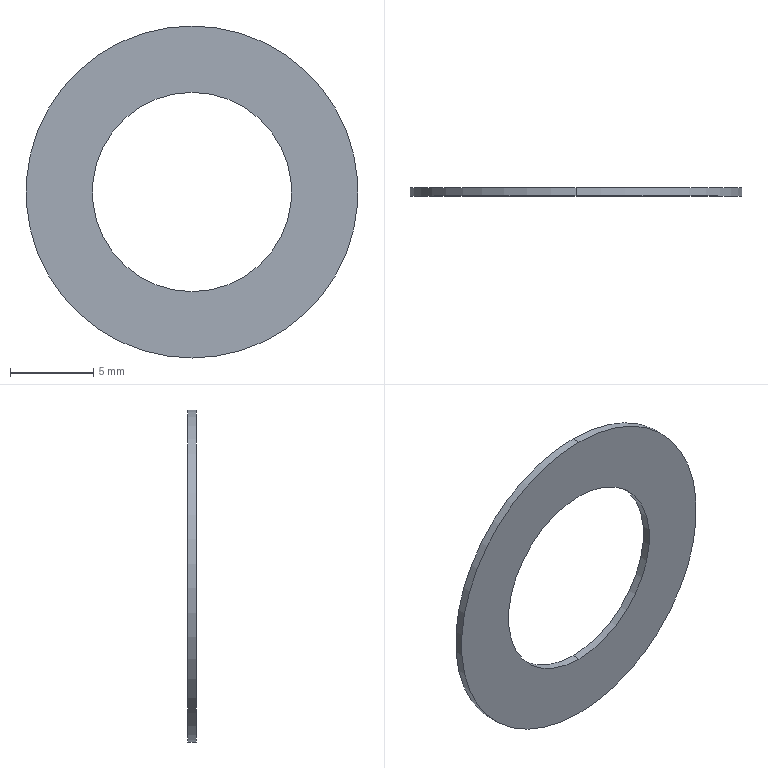Part | SolidWorks | features Extrusion 1 | 1 solid | 6 faces | box 20 x 0.5 x 20 mm | volume 100.531 mm3 | cylinder 4 | plane 2 | commonest cylinder face diameters 12 x2 20 x2
STEP:
#1=CARTESIAN_POINT('',(0.,0.5,-6.));
#2=VERTEX_POINT('',#1);
#3=CARTESIAN_POINT('',(0.,0.5,6.));
#4=VERTEX_POINT('',#3);
#5=CARTESIAN_POINT('',(0.,0.5,0.));
#6=DIRECTION('',(0.,1.,0.));
#7=DIRECTION('',(0.,0.,1.));
#8=AXIS2_PLACEMENT_3D('',#5,#6,#7);
#9=CIRCLE('',#8,6.);
#10=EDGE_CURVE('',#2,#4,#9,.T.);
#11=ORIENTED_EDGE('',*,*,#10,.T.);
#12=CARTESIAN_POINT('',(0.,0.,6.));
#13=VERTEX_POINT('',#12);
#14=CARTESIAN_POINT('',(0.,0.5,6.));
#15=DIRECTION('',(0.,-1.,0.));
#16=VECTOR('',#15,1000.);
#17=LINE('',#14,#16);
#18=EDGE_CURVE('',#4,#13,#17,.T.);
#19=ORIENTED_EDGE('',*,*,#18,.T.);
#20=CARTESIAN_POINT('',(0.,0.,-6.));
#21=VERTEX_POINT('',#20);
#22=CARTESIAN_POINT('',(0.,0.,0.));
#23=DIRECTION('',(0.,1.,0.));
#24=DIRECTION('',(0.,0.,1.));
#25=AXIS2_PLACEMENT_3D('',#22,#23,#24);
#26=CIRCLE('',#25,6.);
#27=EDGE_CURVE('',#21,#13,#26,.T.);
#28=ORIENTED_EDGE('',*,*,#27,.F.);
#29=CARTESIAN_POINT('',(0.,0.5,-6.));
#30=DIRECTION('',(0.,-1.,0.));
#31=VECTOR('',#30,1000.);
#32=LINE('',#29,#31);
#33=EDGE_CURVE('',#2,#21,#32,.T.);
#34=ORIENTED_EDGE('',*,*,#33,.F.);
#35=EDGE_LOOP('',(#11,#19,#28,#34));
#36=FACE_OUTER_BOUND('',#35,.T.);
#37=CARTESIAN_POINT('',(0.,0.5,0.));
#38=DIRECTION('',(0.,-1.,0.));
#39=DIRECTION('',(0.,0.,-1.));
#40=AXIS2_PLACEMENT_3D('',#37,#38,#39);
#41=CYLINDRICAL_SURFACE('',#40,6.);
#42=ADVANCED_FACE('',(#36),#41,.F.);
#43=CARTESIAN_POINT('',(0.,0.5,10.));
#44=VERTEX_POINT('',#43);
#45=CARTESIAN_POINT('',(0.,0.5,-10.));
#46=VERTEX_POINT('',#45);
#47=CARTESIAN_POINT('',(0.,0.5,0.));
#48=DIRECTION('',(0.,1.,0.));
#49=DIRECTION('',(0.,0.,1.));
#50=AXIS2_PLACEMENT_3D('',#47,#48,#49);
#51=CIRCLE('',#50,10.);
#52=EDGE_CURVE('',#44,#46,#51,.T.);
#53=ORIENTED_EDGE('',*,*,#52,.F.);
#54=CARTESIAN_POINT('',(0.,0.,10.));
#55=VERTEX_POINT('',#54);
#56=CARTESIAN_POINT('',(0.,0.5,10.));
#57=DIRECTION('',(0.,-1.,0.));
#58=VECTOR('',#57,1000.);
#59=LINE('',#56,#58);
#60=EDGE_CURVE('',#44,#55,#59,.T.);
#61=ORIENTED_EDGE('',*,*,#60,.T.);
#62=CARTESIAN_POINT('',(0.,0.,-10.));
#63=VERTEX_POINT('',#62);
#64=CARTESIAN_POINT('',(0.,0.,0.));
#65=DIRECTION('',(0.,1.,0.));
#66=DIRECTION('',(0.,0.,1.));
#67=AXIS2_PLACEMENT_3D('',#64,#65,#66);
#68=CIRCLE('',#67,10.);
#69=EDGE_CURVE('',#55,#63,#68,.T.);
#70=ORIENTED_EDGE('',*,*,#69,.T.);
#71=CARTESIAN_POINT('',(0.,0.5,-10.));
#72=DIRECTION('',(0.,-1.,0.));
#73=VECTOR('',#72,1000.);
#74=LINE('',#71,#73);
#75=EDGE_CURVE('',#46,#63,#74,.T.);
#76=ORIENTED_EDGE('',*,*,#75,.F.);
#77=EDGE_LOOP('',(#53,#61,#70,#76));
#78=FACE_OUTER_BOUND('',#77,.T.);
#79=CARTESIAN_POINT('',(0.,0.5,0.));
#80=DIRECTION('',(0.,-1.,0.));
#81=DIRECTION('',(0.,0.,-1.));
#82=AXIS2_PLACEMENT_3D('',#79,#80,#81);
#83=CYLINDRICAL_SURFACE('',#82,10.);
#84=ADVANCED_FACE('',(#78),#83,.T.);
#85=CARTESIAN_POINT('',(0.,0.5,0.));
#86=DIRECTION('',(0.,1.,0.));
#87=DIRECTION('',(0.,0.,1.));
#88=AXIS2_PLACEMENT_3D('',#85,#86,#87);
#89=CIRCLE('',#88,10.);
#90=EDGE_CURVE('',#46,#44,#89,.T.);
#91=ORIENTED_EDGE('',*,*,#90,.T.);
#92=ORIENTED_EDGE('',*,*,#52,.T.);
#93=EDGE_LOOP('',(#91,#92));
#94=FACE_OUTER_BOUND('',#93,.T.);
#95=ORIENTED_EDGE('',*,*,#10,.F.);
#96=CARTESIAN_POINT('',(0.,0.5,0.));
#97=DIRECTION('',(0.,1.,0.));
#98=DIRECTION('',(0.,0.,1.));
#99=AXIS2_PLACEMENT_3D('',#96,#97,#98);
#100=CIRCLE('',#99,6.);
#101=EDGE_CURVE('',#4,#2,#100,.T.);
#102=ORIENTED_EDGE('',*,*,#101,.F.);
#103=EDGE_LOOP('',(#95,#102));
#104=FACE_BOUND('',#103,.T.);
#105=CARTESIAN_POINT('',(0.,0.5,0.));
#106=DIRECTION('',(0.,1.,0.));
#107=DIRECTION('',(0.,0.,1.));
#108=AXIS2_PLACEMENT_3D('',#105,#106,#107);
#109=PLANE('',#108);
#110=ADVANCED_FACE('',(#94,#104),#109,.T.);
#111=CARTESIAN_POINT('',(0.,0.,0.));
#112=DIRECTION('',(0.,1.,0.));
#113=DIRECTION('',(0.,0.,1.));
#114=AXIS2_PLACEMENT_3D('',#111,#112,#113);
#115=CIRCLE('',#114,10.);
#116=EDGE_CURVE('',#63,#55,#115,.T.);
#117=ORIENTED_EDGE('',*,*,#116,.F.);
#118=ORIENTED_EDGE('',*,*,#69,.F.);
#119=EDGE_LOOP('',(#117,#118));
#120=FACE_OUTER_BOUND('',#119,.T.);
#121=ORIENTED_EDGE('',*,*,#27,.T.);
#122=CARTESIAN_POINT('',(0.,0.,0.));
#123=DIRECTION('',(0.,1.,0.));
#124=DIRECTION('',(0.,0.,1.));
#125=AXIS2_PLACEMENT_3D('',#122,#123,#124);
#126=CIRCLE('',#125,6.);
#127=EDGE_CURVE('',#13,#21,#126,.T.);
#128=ORIENTED_EDGE('',*,*,#127,.T.);
#129=EDGE_LOOP('',(#121,#128));
#130=FACE_BOUND('',#129,.T.);
#131=CARTESIAN_POINT('',(0.,0.,0.));
#132=DIRECTION('',(0.,1.,0.));
#133=DIRECTION('',(0.,0.,1.));
#134=AXIS2_PLACEMENT_3D('',#131,#132,#133);
#135=PLANE('',#134);
#136=ADVANCED_FACE('',(#120,#130),#135,.F.);
#137=ORIENTED_EDGE('',*,*,#60,.F.);
#138=ORIENTED_EDGE('',*,*,#90,.F.);
#139=ORIENTED_EDGE('',*,*,#75,.T.);
#140=ORIENTED_EDGE('',*,*,#116,.T.);
#141=EDGE_LOOP('',(#137,#138,#139,#140));
#142=FACE_OUTER_BOUND('',#141,.T.);
#143=CARTESIAN_POINT('',(0.,0.5,0.));
#144=DIRECTION('',(0.,-1.,0.));
#145=DIRECTION('',(0.,0.,-1.));
#146=AXIS2_PLACEMENT_3D('',#143,#144,#145);
#147=CYLINDRICAL_SURFACE('',#146,10.);
#148=ADVANCED_FACE('',(#142),#147,.T.);
#149=ORIENTED_EDGE('',*,*,#18,.F.);
#150=ORIENTED_EDGE('',*,*,#101,.T.);
#151=ORIENTED_EDGE('',*,*,#33,.T.);
#152=ORIENTED_EDGE('',*,*,#127,.F.);
#153=EDGE_LOOP('',(#149,#150,#151,#152));
#154=FACE_OUTER_BOUND('',#153,.T.);
#155=CARTESIAN_POINT('',(0.,0.5,0.));
#156=DIRECTION('',(0.,-1.,0.));
#157=DIRECTION('',(0.,0.,-1.));
#158=AXIS2_PLACEMENT_3D('',#155,#156,#157);
#159=CYLINDRICAL_SURFACE('',#158,6.);
#160=ADVANCED_FACE('',(#154),#159,.F.);
#161=CLOSED_SHELL('',(#42,#84,#110,#136,#148,#160));
#162=MANIFOLD_SOLID_BREP('',#161);
#163=CARTESIAN_POINT('',(0.,0.,0.));
#164=DIRECTION('',(0.,0.,1.));
#165=DIRECTION('',(1.,0.,0.));
#166=AXIS2_PLACEMENT_3D('',#163,#164,#165);
#167=(LENGTH_UNIT()NAMED_UNIT(*)SI_UNIT(.MILLI.,.METRE.));
#168=UNCERTAINTY_MEASURE_WITH_UNIT(LENGTH_MEASURE(0.00001),#167,'','');
#169=(NAMED_UNIT(*)PLANE_ANGLE_UNIT()SI_UNIT($,.RADIAN.));
#170=(NAMED_UNIT(*)SI_UNIT($,.STERADIAN.)SOLID_ANGLE_UNIT());
#171=(GEOMETRIC_REPRESENTATION_CONTEXT(3)GLOBAL_UNCERTAINTY_ASSIGNED_CONTEXT((#168))GLOBAL_UNIT_ASSIGNED_CONTEXT((#167,#169,#170))REPRESENTATION_CONTEXT('',''));
#172=ADVANCED_BREP_SHAPE_REPRESENTATION('',(#162,#166),#171);